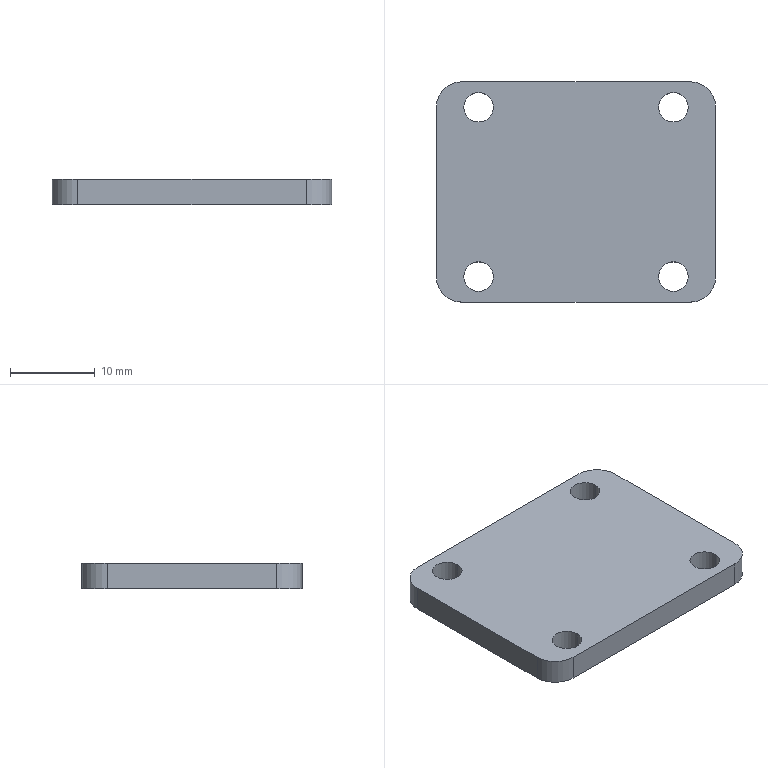Part | SolidWorks | features BaseBody 1 | 1 solid | 18 faces | box 33 x 26 x 3 mm | volume 2435 mm3 | cylinder 12 | plane 6 | commonest cylinder face diameters 3.5 x8 6 x4
STEP:
#1=CARTESIAN_POINT('',(9.75,10.,0.));
#2=VERTEX_POINT('',#1);
#3=CARTESIAN_POINT('',(13.25,10.,0.));
#4=VERTEX_POINT('',#3);
#5=CARTESIAN_POINT('',(11.5,10.,0.));
#6=DIRECTION('',(0.,0.,1.));
#7=DIRECTION('',(1.,0.,0.));
#8=AXIS2_PLACEMENT_3D('',#5,#6,#7);
#9=CIRCLE('',#8,1.75);
#10=EDGE_CURVE('',#2,#4,#9,.T.);
#11=ORIENTED_EDGE('',*,*,#10,.F.);
#12=CARTESIAN_POINT('',(9.75,10.,3.));
#13=VERTEX_POINT('',#12);
#14=CARTESIAN_POINT('',(9.75,10.,3.));
#15=DIRECTION('',(0.,0.,1.));
#16=VECTOR('',#15,1000.);
#17=LINE('',#14,#16);
#18=EDGE_CURVE('',#2,#13,#17,.T.);
#19=ORIENTED_EDGE('',*,*,#18,.T.);
#20=CARTESIAN_POINT('',(13.25,10.,3.));
#21=VERTEX_POINT('',#20);
#22=CARTESIAN_POINT('',(11.5,10.,3.));
#23=DIRECTION('',(0.,0.,-1.));
#24=DIRECTION('',(1.,0.,0.));
#25=AXIS2_PLACEMENT_3D('',#22,#23,#24);
#26=CIRCLE('',#25,1.75);
#27=EDGE_CURVE('',#21,#13,#26,.T.);
#28=ORIENTED_EDGE('',*,*,#27,.F.);
#29=CARTESIAN_POINT('',(13.25,10.,3.));
#30=DIRECTION('',(0.,0.,1.));
#31=VECTOR('',#30,1000.);
#32=LINE('',#29,#31);
#33=EDGE_CURVE('',#4,#21,#32,.T.);
#34=ORIENTED_EDGE('',*,*,#33,.F.);
#35=EDGE_LOOP('',(#11,#19,#28,#34));
#36=FACE_OUTER_BOUND('',#35,.T.);
#37=CARTESIAN_POINT('',(11.5,10.,3.));
#38=DIRECTION('',(0.,0.,1.));
#39=DIRECTION('',(1.,0.,0.));
#40=AXIS2_PLACEMENT_3D('',#37,#38,#39);
#41=CYLINDRICAL_SURFACE('',#40,1.75);
#42=ADVANCED_FACE('',(#36),#41,.F.);
#43=CARTESIAN_POINT('',(9.75,-10.,0.));
#44=VERTEX_POINT('',#43);
#45=CARTESIAN_POINT('',(13.25,-10.,0.));
#46=VERTEX_POINT('',#45);
#47=CARTESIAN_POINT('',(11.5,-10.,0.));
#48=DIRECTION('',(0.,0.,1.));
#49=DIRECTION('',(1.,0.,0.));
#50=AXIS2_PLACEMENT_3D('',#47,#48,#49);
#51=CIRCLE('',#50,1.75);
#52=EDGE_CURVE('',#44,#46,#51,.T.);
#53=ORIENTED_EDGE('',*,*,#52,.F.);
#54=CARTESIAN_POINT('',(9.75,-10.,3.));
#55=VERTEX_POINT('',#54);
#56=CARTESIAN_POINT('',(9.75,-10.,3.));
#57=DIRECTION('',(0.,0.,1.));
#58=VECTOR('',#57,1000.);
#59=LINE('',#56,#58);
#60=EDGE_CURVE('',#44,#55,#59,.T.);
#61=ORIENTED_EDGE('',*,*,#60,.T.);
#62=CARTESIAN_POINT('',(13.25,-10.,3.));
#63=VERTEX_POINT('',#62);
#64=CARTESIAN_POINT('',(11.5,-10.,3.));
#65=DIRECTION('',(0.,0.,-1.));
#66=DIRECTION('',(1.,0.,0.));
#67=AXIS2_PLACEMENT_3D('',#64,#65,#66);
#68=CIRCLE('',#67,1.75);
#69=EDGE_CURVE('',#63,#55,#68,.T.);
#70=ORIENTED_EDGE('',*,*,#69,.F.);
#71=CARTESIAN_POINT('',(13.25,-10.,3.));
#72=DIRECTION('',(0.,0.,1.));
#73=VECTOR('',#72,1000.);
#74=LINE('',#71,#73);
#75=EDGE_CURVE('',#46,#63,#74,.T.);
#76=ORIENTED_EDGE('',*,*,#75,.F.);
#77=EDGE_LOOP('',(#53,#61,#70,#76));
#78=FACE_OUTER_BOUND('',#77,.T.);
#79=CARTESIAN_POINT('',(11.5,-10.,3.));
#80=DIRECTION('',(0.,0.,1.));
#81=DIRECTION('',(1.,0.,0.));
#82=AXIS2_PLACEMENT_3D('',#79,#80,#81);
#83=CYLINDRICAL_SURFACE('',#82,1.75);
#84=ADVANCED_FACE('',(#78),#83,.F.);
#85=CARTESIAN_POINT('',(-13.25,-10.,0.));
#86=VERTEX_POINT('',#85);
#87=CARTESIAN_POINT('',(-9.75,-10.,0.));
#88=VERTEX_POINT('',#87);
#89=CARTESIAN_POINT('',(-11.5,-10.,0.));
#90=DIRECTION('',(0.,0.,1.));
#91=DIRECTION('',(1.,0.,0.));
#92=AXIS2_PLACEMENT_3D('',#89,#90,#91);
#93=CIRCLE('',#92,1.75);
#94=EDGE_CURVE('',#86,#88,#93,.T.);
#95=ORIENTED_EDGE('',*,*,#94,.F.);
#96=CARTESIAN_POINT('',(-13.25,-10.,3.));
#97=VERTEX_POINT('',#96);
#98=CARTESIAN_POINT('',(-13.25,-10.,3.));
#99=DIRECTION('',(0.,0.,1.));
#100=VECTOR('',#99,1000.);
#101=LINE('',#98,#100);
#102=EDGE_CURVE('',#86,#97,#101,.T.);
#103=ORIENTED_EDGE('',*,*,#102,.T.);
#104=CARTESIAN_POINT('',(-9.75,-10.,3.));
#105=VERTEX_POINT('',#104);
#106=CARTESIAN_POINT('',(-11.5,-10.,3.));
#107=DIRECTION('',(0.,0.,-1.));
#108=DIRECTION('',(1.,0.,0.));
#109=AXIS2_PLACEMENT_3D('',#106,#107,#108);
#110=CIRCLE('',#109,1.75);
#111=EDGE_CURVE('',#105,#97,#110,.T.);
#112=ORIENTED_EDGE('',*,*,#111,.F.);
#113=CARTESIAN_POINT('',(-9.75,-10.,3.));
#114=DIRECTION('',(0.,0.,1.));
#115=VECTOR('',#114,1000.);
#116=LINE('',#113,#115);
#117=EDGE_CURVE('',#88,#105,#116,.T.);
#118=ORIENTED_EDGE('',*,*,#117,.F.);
#119=EDGE_LOOP('',(#95,#103,#112,#118));
#120=FACE_OUTER_BOUND('',#119,.T.);
#121=CARTESIAN_POINT('',(-11.5,-10.,3.));
#122=DIRECTION('',(0.,0.,1.));
#123=DIRECTION('',(1.,0.,0.));
#124=AXIS2_PLACEMENT_3D('',#121,#122,#123);
#125=CYLINDRICAL_SURFACE('',#124,1.75);
#126=ADVANCED_FACE('',(#120),#125,.F.);
#127=CARTESIAN_POINT('',(-13.25,10.,0.));
#128=VERTEX_POINT('',#127);
#129=CARTESIAN_POINT('',(-9.75,10.,0.));
#130=VERTEX_POINT('',#129);
#131=CARTESIAN_POINT('',(-11.5,10.,0.));
#132=DIRECTION('',(0.,0.,1.));
#133=DIRECTION('',(1.,0.,0.));
#134=AXIS2_PLACEMENT_3D('',#131,#132,#133);
#135=CIRCLE('',#134,1.75);
#136=EDGE_CURVE('',#128,#130,#135,.T.);
#137=ORIENTED_EDGE('',*,*,#136,.F.);
#138=CARTESIAN_POINT('',(-13.25,10.,3.));
#139=VERTEX_POINT('',#138);
#140=CARTESIAN_POINT('',(-13.25,10.,3.));
#141=DIRECTION('',(0.,0.,1.));
#142=VECTOR('',#141,1000.);
#143=LINE('',#140,#142);
#144=EDGE_CURVE('',#128,#139,#143,.T.);
#145=ORIENTED_EDGE('',*,*,#144,.T.);
#146=CARTESIAN_POINT('',(-9.75,10.,3.));
#147=VERTEX_POINT('',#146);
#148=CARTESIAN_POINT('',(-11.5,10.,3.));
#149=DIRECTION('',(0.,0.,-1.));
#150=DIRECTION('',(1.,0.,0.));
#151=AXIS2_PLACEMENT_3D('',#148,#149,#150);
#152=CIRCLE('',#151,1.75);
#153=EDGE_CURVE('',#147,#139,#152,.T.);
#154=ORIENTED_EDGE('',*,*,#153,.F.);
#155=CARTESIAN_POINT('',(-9.75,10.,3.));
#156=DIRECTION('',(0.,0.,1.));
#157=VECTOR('',#156,1000.);
#158=LINE('',#155,#157);
#159=EDGE_CURVE('',#130,#147,#158,.T.);
#160=ORIENTED_EDGE('',*,*,#159,.F.);
#161=EDGE_LOOP('',(#137,#145,#154,#160));
#162=FACE_OUTER_BOUND('',#161,.T.);
#163=CARTESIAN_POINT('',(-11.5,10.,3.));
#164=DIRECTION('',(0.,0.,1.));
#165=DIRECTION('',(1.,0.,0.));
#166=AXIS2_PLACEMENT_3D('',#163,#164,#165);
#167=CYLINDRICAL_SURFACE('',#166,1.75);
#168=ADVANCED_FACE('',(#162),#167,.F.);
#169=CARTESIAN_POINT('',(16.5,-10.,3.));
#170=VERTEX_POINT('',#169);
#171=CARTESIAN_POINT('',(16.5,10.,3.));
#172=VERTEX_POINT('',#171);
#173=CARTESIAN_POINT('',(16.5,0.,3.));
#174=DIRECTION('',(0.,1.,0.));
#175=VECTOR('',#174,1000.);
#176=LINE('',#173,#175);
#177=EDGE_CURVE('',#170,#172,#176,.T.);
#178=ORIENTED_EDGE('',*,*,#177,.T.);
#179=CARTESIAN_POINT('',(13.5,13.,3.));
#180=VERTEX_POINT('',#179);
#181=CARTESIAN_POINT('',(13.5,10.,3.));
#182=DIRECTION('',(0.,0.,1.));
#183=DIRECTION('',(-1.,0.,0.));
#184=AXIS2_PLACEMENT_3D('',#181,#182,#183);
#185=CIRCLE('',#184,3.);
#186=EDGE_CURVE('',#172,#180,#185,.T.);
#187=ORIENTED_EDGE('',*,*,#186,.T.);
#188=CARTESIAN_POINT('',(-13.5,13.,3.));
#189=VERTEX_POINT('',#188);
#190=CARTESIAN_POINT('',(0.,13.,3.));
#191=DIRECTION('',(-1.,0.,0.));
#192=VECTOR('',#191,1000.);
#193=LINE('',#190,#192);
#194=EDGE_CURVE('',#180,#189,#193,.T.);
#195=ORIENTED_EDGE('',*,*,#194,.T.);
#196=CARTESIAN_POINT('',(-16.5,10.,3.));
#197=VERTEX_POINT('',#196);
#198=CARTESIAN_POINT('',(-13.5,10.,3.));
#199=DIRECTION('',(0.,0.,1.));
#200=DIRECTION('',(-1.,0.,0.));
#201=AXIS2_PLACEMENT_3D('',#198,#199,#200);
#202=CIRCLE('',#201,3.);
#203=EDGE_CURVE('',#189,#197,#202,.T.);
#204=ORIENTED_EDGE('',*,*,#203,.T.);
#205=CARTESIAN_POINT('',(-16.5,-10.,3.));
#206=VERTEX_POINT('',#205);
#207=CARTESIAN_POINT('',(-16.5,0.,3.));
#208=DIRECTION('',(0.,-1.,0.));
#209=VECTOR('',#208,1000.);
#210=LINE('',#207,#209);
#211=EDGE_CURVE('',#197,#206,#210,.T.);
#212=ORIENTED_EDGE('',*,*,#211,.T.);
#213=CARTESIAN_POINT('',(-13.5,-13.,3.));
#214=VERTEX_POINT('',#213);
#215=CARTESIAN_POINT('',(-13.5,-10.,3.));
#216=DIRECTION('',(0.,0.,1.));
#217=DIRECTION('',(-1.,0.,0.));
#218=AXIS2_PLACEMENT_3D('',#215,#216,#217);
#219=CIRCLE('',#218,3.);
#220=EDGE_CURVE('',#206,#214,#219,.T.);
#221=ORIENTED_EDGE('',*,*,#220,.T.);
#222=CARTESIAN_POINT('',(13.5,-13.,3.));
#223=VERTEX_POINT('',#222);
#224=CARTESIAN_POINT('',(0.,-13.,3.));
#225=DIRECTION('',(1.,0.,0.));
#226=VECTOR('',#225,1000.);
#227=LINE('',#224,#226);
#228=EDGE_CURVE('',#214,#223,#227,.T.);
#229=ORIENTED_EDGE('',*,*,#228,.T.);
#230=CARTESIAN_POINT('',(13.5,-10.,3.));
#231=DIRECTION('',(0.,0.,1.));
#232=DIRECTION('',(-1.,0.,0.));
#233=AXIS2_PLACEMENT_3D('',#230,#231,#232);
#234=CIRCLE('',#233,3.);
#235=EDGE_CURVE('',#223,#170,#234,.T.);
#236=ORIENTED_EDGE('',*,*,#235,.T.);
#237=EDGE_LOOP('',(#178,#187,#195,#204,#212,#221,#229,#236));
#238=FACE_OUTER_BOUND('',#237,.T.);
#239=ORIENTED_EDGE('',*,*,#27,.T.);
#240=CARTESIAN_POINT('',(11.5,10.,3.));
#241=DIRECTION('',(0.,0.,-1.));
#242=DIRECTION('',(1.,0.,0.));
#243=AXIS2_PLACEMENT_3D('',#240,#241,#242);
#244=CIRCLE('',#243,1.75);
#245=EDGE_CURVE('',#13,#21,#244,.T.);
#246=ORIENTED_EDGE('',*,*,#245,.T.);
#247=EDGE_LOOP('',(#239,#246));
#248=FACE_BOUND('',#247,.T.);
#249=ORIENTED_EDGE('',*,*,#69,.T.);
#250=CARTESIAN_POINT('',(11.5,-10.,3.));
#251=DIRECTION('',(0.,0.,-1.));
#252=DIRECTION('',(1.,0.,0.));
#253=AXIS2_PLACEMENT_3D('',#250,#251,#252);
#254=CIRCLE('',#253,1.75);
#255=EDGE_CURVE('',#55,#63,#254,.T.);
#256=ORIENTED_EDGE('',*,*,#255,.T.);
#257=EDGE_LOOP('',(#249,#256));
#258=FACE_BOUND('',#257,.T.);
#259=ORIENTED_EDGE('',*,*,#111,.T.);
#260=CARTESIAN_POINT('',(-11.5,-10.,3.));
#261=DIRECTION('',(0.,0.,-1.));
#262=DIRECTION('',(1.,0.,0.));
#263=AXIS2_PLACEMENT_3D('',#260,#261,#262);
#264=CIRCLE('',#263,1.75);
#265=EDGE_CURVE('',#97,#105,#264,.T.);
#266=ORIENTED_EDGE('',*,*,#265,.T.);
#267=EDGE_LOOP('',(#259,#266));
#268=FACE_BOUND('',#267,.T.);
#269=ORIENTED_EDGE('',*,*,#153,.T.);
#270=CARTESIAN_POINT('',(-11.5,10.,3.));
#271=DIRECTION('',(0.,0.,-1.));
#272=DIRECTION('',(1.,0.,0.));
#273=AXIS2_PLACEMENT_3D('',#270,#271,#272);
#274=CIRCLE('',#273,1.75);
#275=EDGE_CURVE('',#139,#147,#274,.T.);
#276=ORIENTED_EDGE('',*,*,#275,.T.);
#277=EDGE_LOOP('',(#269,#276));
#278=FACE_BOUND('',#277,.T.);
#279=CARTESIAN_POINT('',(0.,0.,3.));
#280=DIRECTION('',(0.,0.,1.));
#281=DIRECTION('',(1.,0.,0.));
#282=AXIS2_PLACEMENT_3D('',#279,#280,#281);
#283=PLANE('',#282);
#284=ADVANCED_FACE('',(#238,#248,#258,#268,#278),#283,.T.);
#285=CARTESIAN_POINT('',(16.5,10.,0.));
#286=VERTEX_POINT('',#285);
#287=CARTESIAN_POINT('',(13.5,13.,0.));
#288=VERTEX_POINT('',#287);
#289=CARTESIAN_POINT('',(13.5,10.,0.));
#290=DIRECTION('',(0.,0.,1.));
#291=DIRECTION('',(-1.,0.,0.));
#292=AXIS2_PLACEMENT_3D('',#289,#290,#291);
#293=CIRCLE('',#292,3.);
#294=EDGE_CURVE('',#286,#288,#293,.T.);
#295=ORIENTED_EDGE('',*,*,#294,.T.);
#296=CARTESIAN_POINT('',(13.5,13.,3.));
#297=DIRECTION('',(0.,0.,1.));
#298=VECTOR('',#297,1000.);
#299=LINE('',#296,#298);
#300=EDGE_CURVE('',#288,#180,#299,.T.);
#301=ORIENTED_EDGE('',*,*,#300,.T.);
#302=ORIENTED_EDGE('',*,*,#186,.F.);
#303=CARTESIAN_POINT('',(16.5,10.,3.));
#304=DIRECTION('',(0.,0.,-1.));
#305=VECTOR('',#304,1000.);
#306=LINE('',#303,#305);
#307=EDGE_CURVE('',#172,#286,#306,.T.);
#308=ORIENTED_EDGE('',*,*,#307,.T.);
#309=EDGE_LOOP('',(#295,#301,#302,#308));
#310=FACE_OUTER_BOUND('',#309,.T.);
#311=CARTESIAN_POINT('',(13.5,10.,3.));
#312=DIRECTION('',(0.,0.,-1.));
#313=DIRECTION('',(-1.,0.,0.));
#314=AXIS2_PLACEMENT_3D('',#311,#312,#313);
#315=CYLINDRICAL_SURFACE('',#314,3.);
#316=ADVANCED_FACE('',(#310),#315,.T.);
#317=CARTESIAN_POINT('',(16.5,-10.,0.));
#318=VERTEX_POINT('',#317);
#319=CARTESIAN_POINT('',(16.5,-10.,3.));
#320=DIRECTION('',(0.,0.,1.));
#321=VECTOR('',#320,1000.);
#322=LINE('',#319,#321);
#323=EDGE_CURVE('',#318,#170,#322,.T.);
#324=ORIENTED_EDGE('',*,*,#323,.F.);
#325=CARTESIAN_POINT('',(16.5,-13.,0.));
#326=DIRECTION('',(0.,-1.,0.));
#327=VECTOR('',#326,1000.);
#328=LINE('',#325,#327);
#329=EDGE_CURVE('',#286,#318,#328,.T.);
#330=ORIENTED_EDGE('',*,*,#329,.F.);
#331=ORIENTED_EDGE('',*,*,#307,.F.);
#332=ORIENTED_EDGE('',*,*,#177,.F.);
#333=EDGE_LOOP('',(#324,#330,#331,#332));
#334=FACE_OUTER_BOUND('',#333,.T.);
#335=CARTESIAN_POINT('',(16.5,-13.,3.));
#336=DIRECTION('',(-1.,0.,0.));
#337=DIRECTION('',(0.,0.,1.));
#338=AXIS2_PLACEMENT_3D('',#335,#336,#337);
#339=PLANE('',#338);
#340=ADVANCED_FACE('',(#334),#339,.F.);
#341=CARTESIAN_POINT('',(13.5,-13.,0.));
#342=VERTEX_POINT('',#341);
#343=CARTESIAN_POINT('',(13.5,-10.,0.));
#344=DIRECTION('',(0.,0.,1.));
#345=DIRECTION('',(-1.,0.,0.));
#346=AXIS2_PLACEMENT_3D('',#343,#344,#345);
#347=CIRCLE('',#346,3.);
#348=EDGE_CURVE('',#342,#318,#347,.T.);
#349=ORIENTED_EDGE('',*,*,#348,.T.);
#350=ORIENTED_EDGE('',*,*,#323,.T.);
#351=ORIENTED_EDGE('',*,*,#235,.F.);
#352=CARTESIAN_POINT('',(13.5,-13.,3.));
#353=DIRECTION('',(0.,0.,-1.));
#354=VECTOR('',#353,1000.);
#355=LINE('',#352,#354);
#356=EDGE_CURVE('',#223,#342,#355,.T.);
#357=ORIENTED_EDGE('',*,*,#356,.T.);
#358=EDGE_LOOP('',(#349,#350,#351,#357));
#359=FACE_OUTER_BOUND('',#358,.T.);
#360=CARTESIAN_POINT('',(13.5,-10.,3.));
#361=DIRECTION('',(0.,0.,-1.));
#362=DIRECTION('',(-1.,0.,0.));
#363=AXIS2_PLACEMENT_3D('',#360,#361,#362);
#364=CYLINDRICAL_SURFACE('',#363,3.);
#365=ADVANCED_FACE('',(#359),#364,.T.);
#366=CARTESIAN_POINT('',(-13.5,-13.,0.));
#367=VERTEX_POINT('',#366);
#368=CARTESIAN_POINT('',(-13.5,-13.,3.));
#369=DIRECTION('',(0.,0.,1.));
#370=VECTOR('',#369,1000.);
#371=LINE('',#368,#370);
#372=EDGE_CURVE('',#367,#214,#371,.T.);
#373=ORIENTED_EDGE('',*,*,#372,.F.);
#374=CARTESIAN_POINT('',(16.5,-13.,0.));
#375=DIRECTION('',(-1.,0.,0.));
#376=VECTOR('',#375,1000.);
#377=LINE('',#374,#376);
#378=EDGE_CURVE('',#342,#367,#377,.T.);
#379=ORIENTED_EDGE('',*,*,#378,.F.);
#380=ORIENTED_EDGE('',*,*,#356,.F.);
#381=ORIENTED_EDGE('',*,*,#228,.F.);
#382=EDGE_LOOP('',(#373,#379,#380,#381));
#383=FACE_OUTER_BOUND('',#382,.T.);
#384=CARTESIAN_POINT('',(16.5,-13.,3.));
#385=DIRECTION('',(0.,1.,0.));
#386=DIRECTION('',(-1.,0.,0.));
#387=AXIS2_PLACEMENT_3D('',#384,#385,#386);
#388=PLANE('',#387);
#389=ADVANCED_FACE('',(#383),#388,.F.);
#390=CARTESIAN_POINT('',(-16.5,-10.,0.));
#391=VERTEX_POINT('',#390);
#392=CARTESIAN_POINT('',(-13.5,-10.,0.));
#393=DIRECTION('',(0.,0.,1.));
#394=DIRECTION('',(-1.,0.,0.));
#395=AXIS2_PLACEMENT_3D('',#392,#393,#394);
#396=CIRCLE('',#395,3.);
#397=EDGE_CURVE('',#391,#367,#396,.T.);
#398=ORIENTED_EDGE('',*,*,#397,.T.);
#399=ORIENTED_EDGE('',*,*,#372,.T.);
#400=ORIENTED_EDGE('',*,*,#220,.F.);
#401=CARTESIAN_POINT('',(-16.5,-10.,3.));
#402=DIRECTION('',(0.,0.,-1.));
#403=VECTOR('',#402,1000.);
#404=LINE('',#401,#403);
#405=EDGE_CURVE('',#206,#391,#404,.T.);
#406=ORIENTED_EDGE('',*,*,#405,.T.);
#407=EDGE_LOOP('',(#398,#399,#400,#406));
#408=FACE_OUTER_BOUND('',#407,.T.);
#409=CARTESIAN_POINT('',(-13.5,-10.,3.));
#410=DIRECTION('',(0.,0.,-1.));
#411=DIRECTION('',(-1.,0.,0.));
#412=AXIS2_PLACEMENT_3D('',#409,#410,#411);
#413=CYLINDRICAL_SURFACE('',#412,3.);
#414=ADVANCED_FACE('',(#408),#413,.T.);
#415=CARTESIAN_POINT('',(-16.5,10.,0.));
#416=VERTEX_POINT('',#415);
#417=CARTESIAN_POINT('',(-16.5,10.,3.));
#418=DIRECTION('',(0.,0.,1.));
#419=VECTOR('',#418,1000.);
#420=LINE('',#417,#419);
#421=EDGE_CURVE('',#416,#197,#420,.T.);
#422=ORIENTED_EDGE('',*,*,#421,.F.);
#423=CARTESIAN_POINT('',(-16.5,-13.,0.));
#424=DIRECTION('',(0.,1.,0.));
#425=VECTOR('',#424,1000.);
#426=LINE('',#423,#425);
#427=EDGE_CURVE('',#391,#416,#426,.T.);
#428=ORIENTED_EDGE('',*,*,#427,.F.);
#429=ORIENTED_EDGE('',*,*,#405,.F.);
#430=ORIENTED_EDGE('',*,*,#211,.F.);
#431=EDGE_LOOP('',(#422,#428,#429,#430));
#432=FACE_OUTER_BOUND('',#431,.T.);
#433=CARTESIAN_POINT('',(-16.5,-13.,3.));
#434=DIRECTION('',(1.,0.,0.));
#435=DIRECTION('',(0.,0.,-1.));
#436=AXIS2_PLACEMENT_3D('',#433,#434,#435);
#437=PLANE('',#436);
#438=ADVANCED_FACE('',(#432),#437,.F.);
#439=CARTESIAN_POINT('',(-13.5,13.,0.));
#440=VERTEX_POINT('',#439);
#441=CARTESIAN_POINT('',(-13.5,10.,0.));
#442=DIRECTION('',(0.,0.,1.));
#443=DIRECTION('',(-1.,0.,0.));
#444=AXIS2_PLACEMENT_3D('',#441,#442,#443);
#445=CIRCLE('',#444,3.);
#446=EDGE_CURVE('',#440,#416,#445,.T.);
#447=ORIENTED_EDGE('',*,*,#446,.T.);
#448=ORIENTED_EDGE('',*,*,#421,.T.);
#449=ORIENTED_EDGE('',*,*,#203,.F.);
#450=CARTESIAN_POINT('',(-13.5,13.,3.));
#451=DIRECTION('',(0.,0.,-1.));
#452=VECTOR('',#451,1000.);
#453=LINE('',#450,#452);
#454=EDGE_CURVE('',#189,#440,#453,.T.);
#455=ORIENTED_EDGE('',*,*,#454,.T.);
#456=EDGE_LOOP('',(#447,#448,#449,#455));
#457=FACE_OUTER_BOUND('',#456,.T.);
#458=CARTESIAN_POINT('',(-13.5,10.,3.));
#459=DIRECTION('',(0.,0.,-1.));
#460=DIRECTION('',(-1.,0.,0.));
#461=AXIS2_PLACEMENT_3D('',#458,#459,#460);
#462=CYLINDRICAL_SURFACE('',#461,3.);
#463=ADVANCED_FACE('',(#457),#462,.T.);
#464=ORIENTED_EDGE('',*,*,#454,.F.);
#465=ORIENTED_EDGE('',*,*,#194,.F.);
#466=ORIENTED_EDGE('',*,*,#300,.F.);
#467=CARTESIAN_POINT('',(16.5,13.,0.));
#468=DIRECTION('',(1.,0.,0.));
#469=VECTOR('',#468,1000.);
#470=LINE('',#467,#469);
#471=EDGE_CURVE('',#440,#288,#470,.T.);
#472=ORIENTED_EDGE('',*,*,#471,.F.);
#473=EDGE_LOOP('',(#464,#465,#466,#472));
#474=FACE_OUTER_BOUND('',#473,.T.);
#475=CARTESIAN_POINT('',(16.5,13.,3.));
#476=DIRECTION('',(0.,-1.,0.));
#477=DIRECTION('',(1.,0.,0.));
#478=AXIS2_PLACEMENT_3D('',#475,#476,#477);
#479=PLANE('',#478);
#480=ADVANCED_FACE('',(#474),#479,.F.);
#481=ORIENTED_EDGE('',*,*,#18,.F.);
#482=CARTESIAN_POINT('',(11.5,10.,0.));
#483=DIRECTION('',(0.,0.,1.));
#484=DIRECTION('',(1.,0.,0.));
#485=AXIS2_PLACEMENT_3D('',#482,#483,#484);
#486=CIRCLE('',#485,1.75);
#487=EDGE_CURVE('',#4,#2,#486,.T.);
#488=ORIENTED_EDGE('',*,*,#487,.F.);
#489=ORIENTED_EDGE('',*,*,#33,.T.);
#490=ORIENTED_EDGE('',*,*,#245,.F.);
#491=EDGE_LOOP('',(#481,#488,#489,#490));
#492=FACE_OUTER_BOUND('',#491,.T.);
#493=CARTESIAN_POINT('',(11.5,10.,3.));
#494=DIRECTION('',(0.,0.,1.));
#495=DIRECTION('',(1.,0.,0.));
#496=AXIS2_PLACEMENT_3D('',#493,#494,#495);
#497=CYLINDRICAL_SURFACE('',#496,1.75);
#498=ADVANCED_FACE('',(#492),#497,.F.);
#499=ORIENTED_EDGE('',*,*,#60,.F.);
#500=CARTESIAN_POINT('',(11.5,-10.,0.));
#501=DIRECTION('',(0.,0.,1.));
#502=DIRECTION('',(1.,0.,0.));
#503=AXIS2_PLACEMENT_3D('',#500,#501,#502);
#504=CIRCLE('',#503,1.75);
#505=EDGE_CURVE('',#46,#44,#504,.T.);
#506=ORIENTED_EDGE('',*,*,#505,.F.);
#507=ORIENTED_EDGE('',*,*,#75,.T.);
#508=ORIENTED_EDGE('',*,*,#255,.F.);
#509=EDGE_LOOP('',(#499,#506,#507,#508));
#510=FACE_OUTER_BOUND('',#509,.T.);
#511=CARTESIAN_POINT('',(11.5,-10.,3.));
#512=DIRECTION('',(0.,0.,1.));
#513=DIRECTION('',(1.,0.,0.));
#514=AXIS2_PLACEMENT_3D('',#511,#512,#513);
#515=CYLINDRICAL_SURFACE('',#514,1.75);
#516=ADVANCED_FACE('',(#510),#515,.F.);
#517=ORIENTED_EDGE('',*,*,#102,.F.);
#518=CARTESIAN_POINT('',(-11.5,-10.,0.));
#519=DIRECTION('',(0.,0.,1.));
#520=DIRECTION('',(1.,0.,0.));
#521=AXIS2_PLACEMENT_3D('',#518,#519,#520);
#522=CIRCLE('',#521,1.75);
#523=EDGE_CURVE('',#88,#86,#522,.T.);
#524=ORIENTED_EDGE('',*,*,#523,.F.);
#525=ORIENTED_EDGE('',*,*,#117,.T.);
#526=ORIENTED_EDGE('',*,*,#265,.F.);
#527=EDGE_LOOP('',(#517,#524,#525,#526));
#528=FACE_OUTER_BOUND('',#527,.T.);
#529=CARTESIAN_POINT('',(-11.5,-10.,3.));
#530=DIRECTION('',(0.,0.,1.));
#531=DIRECTION('',(1.,0.,0.));
#532=AXIS2_PLACEMENT_3D('',#529,#530,#531);
#533=CYLINDRICAL_SURFACE('',#532,1.75);
#534=ADVANCED_FACE('',(#528),#533,.F.);
#535=ORIENTED_EDGE('',*,*,#144,.F.);
#536=CARTESIAN_POINT('',(-11.5,10.,0.));
#537=DIRECTION('',(0.,0.,1.));
#538=DIRECTION('',(1.,0.,0.));
#539=AXIS2_PLACEMENT_3D('',#536,#537,#538);
#540=CIRCLE('',#539,1.75);
#541=EDGE_CURVE('',#130,#128,#540,.T.);
#542=ORIENTED_EDGE('',*,*,#541,.F.);
#543=ORIENTED_EDGE('',*,*,#159,.T.);
#544=ORIENTED_EDGE('',*,*,#275,.F.);
#545=EDGE_LOOP('',(#535,#542,#543,#544));
#546=FACE_OUTER_BOUND('',#545,.T.);
#547=CARTESIAN_POINT('',(-11.5,10.,3.));
#548=DIRECTION('',(0.,0.,1.));
#549=DIRECTION('',(1.,0.,0.));
#550=AXIS2_PLACEMENT_3D('',#547,#548,#549);
#551=CYLINDRICAL_SURFACE('',#550,1.75);
#552=ADVANCED_FACE('',(#546),#551,.F.);
#553=ORIENTED_EDGE('',*,*,#446,.F.);
#554=ORIENTED_EDGE('',*,*,#471,.T.);
#555=ORIENTED_EDGE('',*,*,#294,.F.);
#556=ORIENTED_EDGE('',*,*,#329,.T.);
#557=ORIENTED_EDGE('',*,*,#348,.F.);
#558=ORIENTED_EDGE('',*,*,#378,.T.);
#559=ORIENTED_EDGE('',*,*,#397,.F.);
#560=ORIENTED_EDGE('',*,*,#427,.T.);
#561=EDGE_LOOP('',(#553,#554,#555,#556,#557,#558,#559,#560));
#562=FACE_OUTER_BOUND('',#561,.T.);
#563=ORIENTED_EDGE('',*,*,#487,.T.);
#564=ORIENTED_EDGE('',*,*,#10,.T.);
#565=EDGE_LOOP('',(#563,#564));
#566=FACE_BOUND('',#565,.T.);
#567=ORIENTED_EDGE('',*,*,#505,.T.);
#568=ORIENTED_EDGE('',*,*,#52,.T.);
#569=EDGE_LOOP('',(#567,#568));
#570=FACE_BOUND('',#569,.T.);
#571=ORIENTED_EDGE('',*,*,#523,.T.);
#572=ORIENTED_EDGE('',*,*,#94,.T.);
#573=EDGE_LOOP('',(#571,#572));
#574=FACE_BOUND('',#573,.T.);
#575=ORIENTED_EDGE('',*,*,#541,.T.);
#576=ORIENTED_EDGE('',*,*,#136,.T.);
#577=EDGE_LOOP('',(#575,#576));
#578=FACE_BOUND('',#577,.T.);
#579=CARTESIAN_POINT('',(0.,0.,0.));
#580=DIRECTION('',(0.,0.,1.));
#581=DIRECTION('',(1.,0.,0.));
#582=AXIS2_PLACEMENT_3D('',#579,#580,#581);
#583=PLANE('',#582);
#584=ADVANCED_FACE('',(#562,#566,#570,#574,#578),#583,.F.);
#585=CLOSED_SHELL('',(#42,#84,#126,#168,#284,#316,#340,#365,#389,#414,#438,#463,#480,#498,#516,#534,#552,#584));
#586=MANIFOLD_SOLID_BREP('',#585);
#587=CARTESIAN_POINT('',(0.,0.,0.));
#588=DIRECTION('',(0.,0.,1.));
#589=DIRECTION('',(1.,0.,0.));
#590=AXIS2_PLACEMENT_3D('',#587,#588,#589);
#591=(LENGTH_UNIT()NAMED_UNIT(*)SI_UNIT(.MILLI.,.METRE.));
#592=UNCERTAINTY_MEASURE_WITH_UNIT(LENGTH_MEASURE(0.00001),#591,'','');
#593=(NAMED_UNIT(*)PLANE_ANGLE_UNIT()SI_UNIT($,.RADIAN.));
#594=(NAMED_UNIT(*)SI_UNIT($,.STERADIAN.)SOLID_ANGLE_UNIT());
#595=(GEOMETRIC_REPRESENTATION_CONTEXT(3)GLOBAL_UNCERTAINTY_ASSIGNED_CONTEXT((#592))GLOBAL_UNIT_ASSIGNED_CONTEXT((#591,#593,#594))REPRESENTATION_CONTEXT('',''));
#596=ADVANCED_BREP_SHAPE_REPRESENTATION('',(#586,#590),#595);